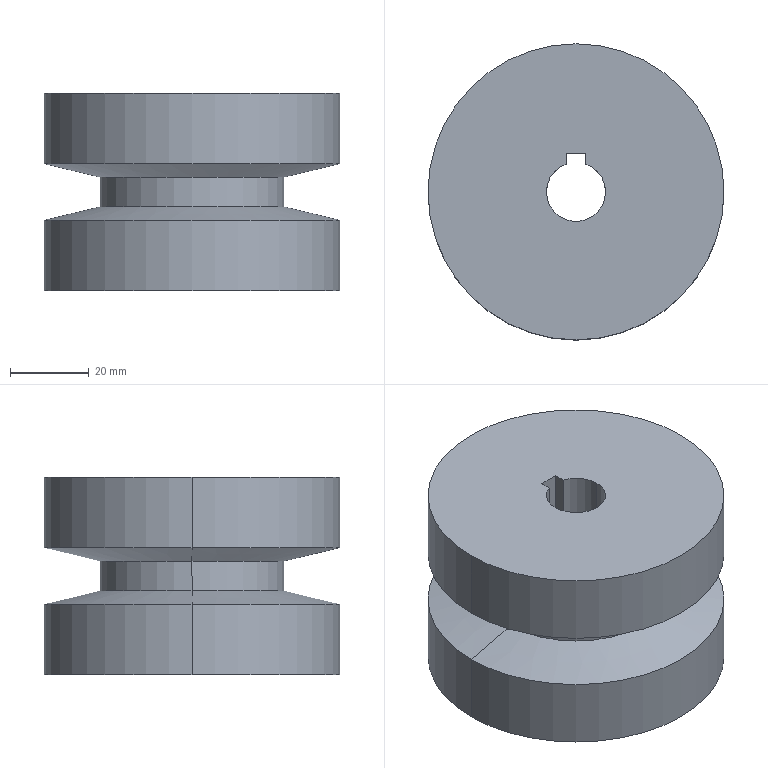Part | SolidWorks | features HoleWzd 2, Extrusion 1, ICE 1, RevCut 1 | 1 solid | 24 faces | box 75 x 75 x 50 mm | volume 180356 mm3 | cylinder 13 | plane 7 | cone 4 | commonest cylinder face diameters 4.2 x4 75 x4 15 x3 46.5 x2
STEP:
#1=CARTESIAN_POINT('',(0.,9.8,11.1));
#2=VERTEX_POINT('',#1);
#3=CARTESIAN_POINT('',(0.,9.8,6.9));
#4=VERTEX_POINT('',#3);
#5=CARTESIAN_POINT('',(0.,9.8,9.));
#6=DIRECTION('',(0.,-1.,0.));
#7=DIRECTION('',(0.,0.,1.));
#8=AXIS2_PLACEMENT_3D('',#5,#6,#7);
#9=CIRCLE('',#8,2.1);
#10=EDGE_CURVE('',#2,#4,#9,.T.);
#11=ORIENTED_EDGE('',*,*,#10,.T.);
#12=CARTESIAN_POINT('',(0.,32.5,6.9));
#13=VERTEX_POINT('',#12);
#14=CARTESIAN_POINT('',(0.,32.5,6.9));
#15=DIRECTION('',(0.,1.,0.));
#16=VECTOR('',#15,1000.);
#17=LINE('',#14,#16);
#18=EDGE_CURVE('',#4,#13,#17,.T.);
#19=ORIENTED_EDGE('',*,*,#18,.T.);
#20=CARTESIAN_POINT('',(0.,32.5,11.1));
#21=VERTEX_POINT('',#20);
#22=CARTESIAN_POINT('',(0.,32.5,9.));
#23=DIRECTION('',(0.,1.,0.));
#24=DIRECTION('',(0.,0.,1.));
#25=AXIS2_PLACEMENT_3D('',#22,#23,#24);
#26=CIRCLE('',#25,2.1);
#27=EDGE_CURVE('',#13,#21,#26,.T.);
#28=ORIENTED_EDGE('',*,*,#27,.T.);
#29=CARTESIAN_POINT('',(0.,32.5,11.1));
#30=DIRECTION('',(0.,1.,0.));
#31=VECTOR('',#30,1000.);
#32=LINE('',#29,#31);
#33=EDGE_CURVE('',#2,#21,#32,.T.);
#34=ORIENTED_EDGE('',*,*,#33,.F.);
#35=EDGE_LOOP('',(#11,#19,#28,#34));
#36=FACE_OUTER_BOUND('',#35,.T.);
#37=CARTESIAN_POINT('',(0.,32.5,9.));
#38=DIRECTION('',(0.,1.,0.));
#39=DIRECTION('',(0.,0.,1.));
#40=AXIS2_PLACEMENT_3D('',#37,#38,#39);
#41=CYLINDRICAL_SURFACE('',#40,2.1);
#42=ADVANCED_FACE('',(#36),#41,.F.);
#43=CARTESIAN_POINT('',(7.5,0.,6.9));
#44=VERTEX_POINT('',#43);
#45=CARTESIAN_POINT('',(7.5,0.,11.1));
#46=VERTEX_POINT('',#45);
#47=CARTESIAN_POINT('',(7.5,0.,6.9));
#48=CARTESIAN_POINT('',(7.5,-0.1395,6.9));
#49=CARTESIAN_POINT('',(7.496,-0.2765,6.914));
#50=CARTESIAN_POINT('',(7.481,-0.5459,6.968));
#51=CARTESIAN_POINT('',(7.47,-0.6797,7.008));
#52=CARTESIAN_POINT('',(7.443,-0.9337,7.114));
#53=CARTESIAN_POINT('',(7.426,-1.054,7.179));
#54=CARTESIAN_POINT('',(7.391,-1.282,7.331));
#55=CARTESIAN_POINT('',(7.371,-1.389,7.419));
#56=CARTESIAN_POINT('',(7.313,-1.678,7.708));
#57=CARTESIAN_POINT('',(7.273,-1.834,7.941));
#58=CARTESIAN_POINT('',(7.231,-1.992,8.32));
#59=CARTESIAN_POINT('',(7.219,-2.032,8.453));
#60=CARTESIAN_POINT('',(7.204,-2.086,8.725));
#61=CARTESIAN_POINT('',(7.2,-2.1,8.861));
#62=CARTESIAN_POINT('',(7.2,-2.1,9.137));
#63=CARTESIAN_POINT('',(7.204,-2.086,9.277));
#64=CARTESIAN_POINT('',(7.219,-2.032,9.547));
#65=CARTESIAN_POINT('',(7.231,-1.992,9.678));
#66=CARTESIAN_POINT('',(7.273,-1.833,10.061));
#67=CARTESIAN_POINT('',(7.312,-1.679,10.291));
#68=CARTESIAN_POINT('',(7.371,-1.387,10.582));
#69=CARTESIAN_POINT('',(7.39,-1.282,10.669));
#70=CARTESIAN_POINT('',(7.426,-1.055,10.821));
#71=CARTESIAN_POINT('',(7.443,-0.9321,10.887));
#72=CARTESIAN_POINT('',(7.47,-0.6788,10.992));
#73=CARTESIAN_POINT('',(7.481,-0.5478,11.032));
#74=CARTESIAN_POINT('',(7.496,-0.2769,11.086));
#75=CARTESIAN_POINT('',(7.5,-0.1375,11.1));
#76=CARTESIAN_POINT('',(7.5,0.,11.1));
#77=B_SPLINE_CURVE_WITH_KNOTS('',3,(#47,#48,#49,#50,#51,#52,#53,#54,#55,#56,#57,#58,#59,#60,#61,#62,#63,#64,#65,#66,#67,#68,#69,#70,#71,#72,#73,#74,#75,#76),.UNSPECIFIED.,.F.,.F.,(4,2,2,2,2,2,2,2,2,2,2,2,2,2,4),(0.,0.0004124,0.0008248,0.001237,0.00165,0.002475,0.002887,0.003299,0.003712,0.004124,0.004949,0.005361,0.005774,0.006186,0.006599),.UNSPECIFIED.);
#78=EDGE_CURVE('',#44,#46,#77,.T.);
#79=ORIENTED_EDGE('',*,*,#78,.T.);
#80=CARTESIAN_POINT('',(32.5,0.,11.1));
#81=VERTEX_POINT('',#80);
#82=CARTESIAN_POINT('',(32.5,0.,11.1));
#83=DIRECTION('',(1.,0.,0.));
#84=VECTOR('',#83,1000.);
#85=LINE('',#82,#84);
#86=EDGE_CURVE('',#46,#81,#85,.T.);
#87=ORIENTED_EDGE('',*,*,#86,.T.);
#88=CARTESIAN_POINT('',(32.5,0.,6.9));
#89=VERTEX_POINT('',#88);
#90=CARTESIAN_POINT('',(32.5,0.,9.));
#91=DIRECTION('',(1.,0.,0.));
#92=DIRECTION('',(0.,0.,-1.));
#93=AXIS2_PLACEMENT_3D('',#90,#91,#92);
#94=CIRCLE('',#93,2.1);
#95=EDGE_CURVE('',#81,#89,#94,.T.);
#96=ORIENTED_EDGE('',*,*,#95,.T.);
#97=CARTESIAN_POINT('',(32.5,0.,6.9));
#98=DIRECTION('',(1.,0.,0.));
#99=VECTOR('',#98,1000.);
#100=LINE('',#97,#99);
#101=EDGE_CURVE('',#44,#89,#100,.T.);
#102=ORIENTED_EDGE('',*,*,#101,.F.);
#103=EDGE_LOOP('',(#79,#87,#96,#102));
#104=FACE_OUTER_BOUND('',#103,.T.);
#105=CARTESIAN_POINT('',(32.5,0.,9.));
#106=DIRECTION('',(1.,0.,0.));
#107=DIRECTION('',(0.,0.,-1.));
#108=AXIS2_PLACEMENT_3D('',#105,#106,#107);
#109=CYLINDRICAL_SURFACE('',#108,2.1);
#110=ADVANCED_FACE('',(#104),#109,.F.);
#111=CARTESIAN_POINT('',(-23.25,0.,28.75));
#112=VERTEX_POINT('',#111);
#113=CARTESIAN_POINT('',(23.25,0.,28.75));
#114=VERTEX_POINT('',#113);
#115=CARTESIAN_POINT('',(0.,0.,28.75));
#116=DIRECTION('',(0.,0.,-1.));
#117=DIRECTION('',(-1.,0.,0.));
#118=AXIS2_PLACEMENT_3D('',#115,#116,#117);
#119=CIRCLE('',#118,23.25);
#120=EDGE_CURVE('',#112,#114,#119,.T.);
#121=ORIENTED_EDGE('',*,*,#120,.T.);
#122=CARTESIAN_POINT('',(23.25,0.,21.25));
#123=VERTEX_POINT('',#122);
#124=CARTESIAN_POINT('',(23.25,0.,0.));
#125=DIRECTION('',(0.,0.,-1.));
#126=VECTOR('',#125,1000.);
#127=LINE('',#124,#126);
#128=EDGE_CURVE('',#114,#123,#127,.T.);
#129=ORIENTED_EDGE('',*,*,#128,.T.);
#130=CARTESIAN_POINT('',(-23.25,0.,21.25));
#131=VERTEX_POINT('',#130);
#132=CARTESIAN_POINT('',(0.,0.,21.25));
#133=DIRECTION('',(0.,0.,-1.));
#134=DIRECTION('',(-1.,0.,0.));
#135=AXIS2_PLACEMENT_3D('',#132,#133,#134);
#136=CIRCLE('',#135,23.25);
#137=EDGE_CURVE('',#131,#123,#136,.T.);
#138=ORIENTED_EDGE('',*,*,#137,.F.);
#139=CARTESIAN_POINT('',(-23.25,0.,0.));
#140=DIRECTION('',(0.,0.,-1.));
#141=VECTOR('',#140,1000.);
#142=LINE('',#139,#141);
#143=EDGE_CURVE('',#112,#131,#142,.T.);
#144=ORIENTED_EDGE('',*,*,#143,.F.);
#145=EDGE_LOOP('',(#121,#129,#138,#144));
#146=FACE_OUTER_BOUND('',#145,.T.);
#147=CARTESIAN_POINT('',(0.,0.,0.));
#148=DIRECTION('',(0.,0.,-1.));
#149=DIRECTION('',(-1.,0.,0.));
#150=AXIS2_PLACEMENT_3D('',#147,#148,#149);
#151=CYLINDRICAL_SURFACE('',#150,23.25);
#152=ADVANCED_FACE('',(#146),#151,.T.);
#153=ORIENTED_EDGE('',*,*,#120,.F.);
#154=CARTESIAN_POINT('',(-37.5,0.,32.171));
#155=VERTEX_POINT('',#154);
#156=CARTESIAN_POINT('',(-38.25,0.,32.351));
#157=DIRECTION('',(-0.9724,0.,0.2334));
#158=VECTOR('',#157,1000.);
#159=LINE('',#156,#158);
#160=EDGE_CURVE('',#112,#155,#159,.T.);
#161=ORIENTED_EDGE('',*,*,#160,.T.);
#162=CARTESIAN_POINT('',(37.5,0.,32.171));
#163=VERTEX_POINT('',#162);
#164=CARTESIAN_POINT('',(0.,0.,32.171));
#165=DIRECTION('',(0.,0.,1.));
#166=DIRECTION('',(1.,0.,0.));
#167=AXIS2_PLACEMENT_3D('',#164,#165,#166);
#168=CIRCLE('',#167,37.5);
#169=EDGE_CURVE('',#163,#155,#168,.T.);
#170=ORIENTED_EDGE('',*,*,#169,.F.);
#171=CARTESIAN_POINT('',(38.25,0.,32.351));
#172=DIRECTION('',(0.9724,0.,0.2334));
#173=VECTOR('',#172,1000.);
#174=LINE('',#171,#173);
#175=EDGE_CURVE('',#114,#163,#174,.T.);
#176=ORIENTED_EDGE('',*,*,#175,.F.);
#177=EDGE_LOOP('',(#153,#161,#170,#176));
#178=FACE_OUTER_BOUND('',#177,.T.);
#179=CARTESIAN_POINT('',(0.,0.,32.351));
#180=DIRECTION('',(0.,0.,1.));
#181=DIRECTION('',(1.,0.,0.));
#182=AXIS2_PLACEMENT_3D('',#179,#180,#181);
#183=CONICAL_SURFACE('',#182,38.25,1.335);
#184=ADVANCED_FACE('',(#178),#183,.T.);
#185=ORIENTED_EDGE('',*,*,#137,.T.);
#186=CARTESIAN_POINT('',(37.5,0.,17.829));
#187=VERTEX_POINT('',#186);
#188=CARTESIAN_POINT('',(23.25,0.,21.25));
#189=DIRECTION('',(0.9724,0.,-0.2334));
#190=VECTOR('',#189,1000.);
#191=LINE('',#188,#190);
#192=EDGE_CURVE('',#123,#187,#191,.T.);
#193=ORIENTED_EDGE('',*,*,#192,.T.);
#194=CARTESIAN_POINT('',(-37.5,0.,17.829));
#195=VERTEX_POINT('',#194);
#196=CARTESIAN_POINT('',(0.,0.,17.829));
#197=DIRECTION('',(0.,0.,-1.));
#198=DIRECTION('',(-1.,0.,0.));
#199=AXIS2_PLACEMENT_3D('',#196,#197,#198);
#200=CIRCLE('',#199,37.5);
#201=EDGE_CURVE('',#195,#187,#200,.T.);
#202=ORIENTED_EDGE('',*,*,#201,.F.);
#203=CARTESIAN_POINT('',(-23.25,0.,21.25));
#204=DIRECTION('',(-0.9724,0.,-0.2334));
#205=VECTOR('',#204,1000.);
#206=LINE('',#203,#205);
#207=EDGE_CURVE('',#131,#195,#206,.T.);
#208=ORIENTED_EDGE('',*,*,#207,.F.);
#209=EDGE_LOOP('',(#185,#193,#202,#208));
#210=FACE_OUTER_BOUND('',#209,.T.);
#211=CARTESIAN_POINT('',(0.,0.,21.25));
#212=DIRECTION('',(0.,0.,-1.));
#213=DIRECTION('',(-1.,0.,0.));
#214=AXIS2_PLACEMENT_3D('',#211,#212,#213);
#215=CONICAL_SURFACE('',#214,23.25,1.335);
#216=ADVANCED_FACE('',(#210),#215,.T.);
#217=CARTESIAN_POINT('',(-7.5,0.,50.));
#218=VERTEX_POINT('',#217);
#219=CARTESIAN_POINT('',(7.5,0.,50.));
#220=VERTEX_POINT('',#219);
#221=CARTESIAN_POINT('',(0.,0.,50.));
#222=DIRECTION('',(0.,0.,1.));
#223=DIRECTION('',(1.,0.,0.));
#224=AXIS2_PLACEMENT_3D('',#221,#222,#223);
#225=CIRCLE('',#224,7.5);
#226=EDGE_CURVE('',#218,#220,#225,.T.);
#227=ORIENTED_EDGE('',*,*,#226,.T.);
#228=CARTESIAN_POINT('',(7.5,0.,50.));
#229=DIRECTION('',(0.,0.,-1.));
#230=VECTOR('',#229,1000.);
#231=LINE('',#228,#230);
#232=EDGE_CURVE('',#220,#46,#231,.T.);
#233=ORIENTED_EDGE('',*,*,#232,.T.);
#234=ORIENTED_EDGE('',*,*,#78,.F.);
#235=CARTESIAN_POINT('',(7.5,0.,0.));
#236=VERTEX_POINT('',#235);
#237=CARTESIAN_POINT('',(7.5,0.,50.));
#238=DIRECTION('',(0.,0.,-1.));
#239=VECTOR('',#238,1000.);
#240=LINE('',#237,#239);
#241=EDGE_CURVE('',#44,#236,#240,.T.);
#242=ORIENTED_EDGE('',*,*,#241,.T.);
#243=CARTESIAN_POINT('',(-7.5,0.,0.));
#244=VERTEX_POINT('',#243);
#245=CARTESIAN_POINT('',(0.,0.,0.));
#246=DIRECTION('',(0.,0.,1.));
#247=DIRECTION('',(1.,0.,0.));
#248=AXIS2_PLACEMENT_3D('',#245,#246,#247);
#249=CIRCLE('',#248,7.5);
#250=EDGE_CURVE('',#244,#236,#249,.T.);
#251=ORIENTED_EDGE('',*,*,#250,.F.);
#252=CARTESIAN_POINT('',(-7.5,0.,50.));
#253=DIRECTION('',(0.,0.,-1.));
#254=VECTOR('',#253,1000.);
#255=LINE('',#252,#254);
#256=EDGE_CURVE('',#218,#244,#255,.T.);
#257=ORIENTED_EDGE('',*,*,#256,.F.);
#258=EDGE_LOOP('',(#227,#233,#234,#242,#251,#257));
#259=FACE_OUTER_BOUND('',#258,.T.);
#260=CARTESIAN_POINT('',(0.,0.,50.));
#261=DIRECTION('',(0.,0.,-1.));
#262=DIRECTION('',(-1.,0.,0.));
#263=AXIS2_PLACEMENT_3D('',#260,#261,#262);
#264=CYLINDRICAL_SURFACE('',#263,7.5);
#265=ADVANCED_FACE('',(#259),#264,.F.);
#266=CARTESIAN_POINT('',(-2.5,7.071,50.));
#267=VERTEX_POINT('',#266);
#268=CARTESIAN_POINT('',(0.,0.,50.));
#269=DIRECTION('',(0.,0.,1.));
#270=DIRECTION('',(1.,0.,0.));
#271=AXIS2_PLACEMENT_3D('',#268,#269,#270);
#272=CIRCLE('',#271,7.5);
#273=EDGE_CURVE('',#267,#218,#272,.T.);
#274=ORIENTED_EDGE('',*,*,#273,.T.);
#275=ORIENTED_EDGE('',*,*,#256,.T.);
#276=CARTESIAN_POINT('',(-2.5,7.071,0.));
#277=VERTEX_POINT('',#276);
#278=CARTESIAN_POINT('',(0.,0.,0.));
#279=DIRECTION('',(0.,0.,1.));
#280=DIRECTION('',(1.,0.,0.));
#281=AXIS2_PLACEMENT_3D('',#278,#279,#280);
#282=CIRCLE('',#281,7.5);
#283=EDGE_CURVE('',#277,#244,#282,.T.);
#284=ORIENTED_EDGE('',*,*,#283,.F.);
#285=CARTESIAN_POINT('',(-2.5,7.071,50.));
#286=DIRECTION('',(0.,0.,-1.));
#287=VECTOR('',#286,1000.);
#288=LINE('',#285,#287);
#289=EDGE_CURVE('',#267,#277,#288,.T.);
#290=ORIENTED_EDGE('',*,*,#289,.F.);
#291=EDGE_LOOP('',(#274,#275,#284,#290));
#292=FACE_OUTER_BOUND('',#291,.T.);
#293=CARTESIAN_POINT('',(0.,0.,50.));
#294=DIRECTION('',(0.,0.,-1.));
#295=DIRECTION('',(-1.,0.,0.));
#296=AXIS2_PLACEMENT_3D('',#293,#294,#295);
#297=CYLINDRICAL_SURFACE('',#296,7.5);
#298=ADVANCED_FACE('',(#292),#297,.F.);
#299=CARTESIAN_POINT('',(37.5,0.,50.));
#300=VERTEX_POINT('',#299);
#301=CARTESIAN_POINT('',(-37.5,0.,50.));
#302=VERTEX_POINT('',#301);
#303=CARTESIAN_POINT('',(0.,0.,50.));
#304=DIRECTION('',(0.,0.,1.));
#305=DIRECTION('',(1.,0.,0.));
#306=AXIS2_PLACEMENT_3D('',#303,#304,#305);
#307=CIRCLE('',#306,37.5);
#308=EDGE_CURVE('',#300,#302,#307,.T.);
#309=ORIENTED_EDGE('',*,*,#308,.F.);
#310=CARTESIAN_POINT('',(37.5,0.,50.));
#311=DIRECTION('',(0.,0.,-1.));
#312=VECTOR('',#311,1000.);
#313=LINE('',#310,#312);
#314=EDGE_CURVE('',#300,#163,#313,.T.);
#315=ORIENTED_EDGE('',*,*,#314,.T.);
#316=ORIENTED_EDGE('',*,*,#169,.T.);
#317=CARTESIAN_POINT('',(-37.5,0.,50.));
#318=DIRECTION('',(0.,0.,-1.));
#319=VECTOR('',#318,1000.);
#320=LINE('',#317,#319);
#321=EDGE_CURVE('',#302,#155,#320,.T.);
#322=ORIENTED_EDGE('',*,*,#321,.F.);
#323=EDGE_LOOP('',(#309,#315,#316,#322));
#324=FACE_OUTER_BOUND('',#323,.T.);
#325=CARTESIAN_POINT('',(0.,0.,50.));
#326=DIRECTION('',(0.,0.,-1.));
#327=DIRECTION('',(-1.,0.,0.));
#328=AXIS2_PLACEMENT_3D('',#325,#326,#327);
#329=CYLINDRICAL_SURFACE('',#328,37.5);
#330=ADVANCED_FACE('',(#324),#329,.T.);
#331=ORIENTED_EDGE('',*,*,#201,.T.);
#332=CARTESIAN_POINT('',(37.5,0.,0.));
#333=VERTEX_POINT('',#332);
#334=CARTESIAN_POINT('',(37.5,0.,50.));
#335=DIRECTION('',(0.,0.,-1.));
#336=VECTOR('',#335,1000.);
#337=LINE('',#334,#336);
#338=EDGE_CURVE('',#187,#333,#337,.T.);
#339=ORIENTED_EDGE('',*,*,#338,.T.);
#340=CARTESIAN_POINT('',(-37.5,0.,0.));
#341=VERTEX_POINT('',#340);
#342=CARTESIAN_POINT('',(0.,0.,0.));
#343=DIRECTION('',(0.,0.,1.));
#344=DIRECTION('',(1.,0.,0.));
#345=AXIS2_PLACEMENT_3D('',#342,#343,#344);
#346=CIRCLE('',#345,37.5);
#347=EDGE_CURVE('',#333,#341,#346,.T.);
#348=ORIENTED_EDGE('',*,*,#347,.T.);
#349=CARTESIAN_POINT('',(-37.5,0.,50.));
#350=DIRECTION('',(0.,0.,-1.));
#351=VECTOR('',#350,1000.);
#352=LINE('',#349,#351);
#353=EDGE_CURVE('',#195,#341,#352,.T.);
#354=ORIENTED_EDGE('',*,*,#353,.F.);
#355=EDGE_LOOP('',(#331,#339,#348,#354));
#356=FACE_OUTER_BOUND('',#355,.T.);
#357=CARTESIAN_POINT('',(0.,0.,50.));
#358=DIRECTION('',(0.,0.,-1.));
#359=DIRECTION('',(-1.,0.,0.));
#360=AXIS2_PLACEMENT_3D('',#357,#358,#359);
#361=CYLINDRICAL_SURFACE('',#360,37.5);
#362=ADVANCED_FACE('',(#356),#361,.T.);
#363=ORIENTED_EDGE('',*,*,#338,.F.);
#364=CARTESIAN_POINT('',(0.,0.,17.829));
#365=DIRECTION('',(0.,0.,-1.));
#366=DIRECTION('',(-1.,0.,0.));
#367=AXIS2_PLACEMENT_3D('',#364,#365,#366);
#368=CIRCLE('',#367,37.5);
#369=EDGE_CURVE('',#187,#195,#368,.T.);
#370=ORIENTED_EDGE('',*,*,#369,.T.);
#371=ORIENTED_EDGE('',*,*,#353,.T.);
#372=CARTESIAN_POINT('',(0.,0.,0.));
#373=DIRECTION('',(0.,0.,1.));
#374=DIRECTION('',(1.,0.,0.));
#375=AXIS2_PLACEMENT_3D('',#372,#373,#374);
#376=CIRCLE('',#375,37.5);
#377=EDGE_CURVE('',#341,#333,#376,.T.);
#378=ORIENTED_EDGE('',*,*,#377,.T.);
#379=EDGE_LOOP('',(#363,#370,#371,#378));
#380=FACE_OUTER_BOUND('',#379,.T.);
#381=CARTESIAN_POINT('',(0.,0.,50.));
#382=DIRECTION('',(0.,0.,-1.));
#383=DIRECTION('',(-1.,0.,0.));
#384=AXIS2_PLACEMENT_3D('',#381,#382,#383);
#385=CYLINDRICAL_SURFACE('',#384,37.5);
#386=ADVANCED_FACE('',(#380),#385,.T.);
#387=CARTESIAN_POINT('',(-2.5,9.8,50.));
#388=VERTEX_POINT('',#387);
#389=CARTESIAN_POINT('',(-2.5,0.,50.));
#390=DIRECTION('',(0.,-1.,0.));
#391=VECTOR('',#390,1000.);
#392=LINE('',#389,#391);
#393=EDGE_CURVE('',#388,#267,#392,.T.);
#394=ORIENTED_EDGE('',*,*,#393,.F.);
#395=CARTESIAN_POINT('',(2.5,9.8,50.));
#396=VERTEX_POINT('',#395);
#397=CARTESIAN_POINT('',(0.,9.8,50.));
#398=DIRECTION('',(-1.,0.,0.));
#399=VECTOR('',#398,1000.);
#400=LINE('',#397,#399);
#401=EDGE_CURVE('',#396,#388,#400,.T.);
#402=ORIENTED_EDGE('',*,*,#401,.F.);
#403=CARTESIAN_POINT('',(2.5,7.071,50.));
#404=VERTEX_POINT('',#403);
#405=CARTESIAN_POINT('',(2.5,0.,50.));
#406=DIRECTION('',(0.,1.,0.));
#407=VECTOR('',#406,1000.);
#408=LINE('',#405,#407);
#409=EDGE_CURVE('',#404,#396,#408,.T.);
#410=ORIENTED_EDGE('',*,*,#409,.F.);
#411=CARTESIAN_POINT('',(0.,0.,50.));
#412=DIRECTION('',(0.,0.,1.));
#413=DIRECTION('',(1.,0.,0.));
#414=AXIS2_PLACEMENT_3D('',#411,#412,#413);
#415=CIRCLE('',#414,7.5);
#416=EDGE_CURVE('',#220,#404,#415,.T.);
#417=ORIENTED_EDGE('',*,*,#416,.F.);
#418=ORIENTED_EDGE('',*,*,#226,.F.);
#419=ORIENTED_EDGE('',*,*,#273,.F.);
#420=EDGE_LOOP('',(#394,#402,#410,#417,#418,#419));
#421=FACE_BOUND('',#420,.T.);
#422=CARTESIAN_POINT('',(0.,0.,50.));
#423=DIRECTION('',(0.,0.,1.));
#424=DIRECTION('',(1.,0.,0.));
#425=AXIS2_PLACEMENT_3D('',#422,#423,#424);
#426=CIRCLE('',#425,37.5);
#427=EDGE_CURVE('',#302,#300,#426,.T.);
#428=ORIENTED_EDGE('',*,*,#427,.T.);
#429=ORIENTED_EDGE('',*,*,#308,.T.);
#430=EDGE_LOOP('',(#428,#429));
#431=FACE_OUTER_BOUND('',#430,.T.);
#432=CARTESIAN_POINT('',(0.,0.,50.));
#433=DIRECTION('',(0.,0.,1.));
#434=DIRECTION('',(1.,0.,0.));
#435=AXIS2_PLACEMENT_3D('',#432,#433,#434);
#436=PLANE('',#435);
#437=ADVANCED_FACE('',(#421,#431),#436,.T.);
#438=ORIENTED_EDGE('',*,*,#377,.F.);
#439=ORIENTED_EDGE('',*,*,#347,.F.);
#440=EDGE_LOOP('',(#438,#439));
#441=FACE_OUTER_BOUND('',#440,.T.);
#442=CARTESIAN_POINT('',(-2.5,9.8,0.));
#443=VERTEX_POINT('',#442);
#444=CARTESIAN_POINT('',(2.5,9.8,0.));
#445=VERTEX_POINT('',#444);
#446=CARTESIAN_POINT('',(2.5,9.8,0.));
#447=DIRECTION('',(1.,0.,0.));
#448=VECTOR('',#447,1000.);
#449=LINE('',#446,#448);
#450=EDGE_CURVE('',#443,#445,#449,.T.);
#451=ORIENTED_EDGE('',*,*,#450,.F.);
#452=CARTESIAN_POINT('',(-2.5,5.2,0.));
#453=DIRECTION('',(0.,1.,0.));
#454=VECTOR('',#453,1000.);
#455=LINE('',#452,#454);
#456=EDGE_CURVE('',#277,#443,#455,.T.);
#457=ORIENTED_EDGE('',*,*,#456,.F.);
#458=ORIENTED_EDGE('',*,*,#283,.T.);
#459=ORIENTED_EDGE('',*,*,#250,.T.);
#460=CARTESIAN_POINT('',(2.5,7.071,0.));
#461=VERTEX_POINT('',#460);
#462=CARTESIAN_POINT('',(0.,0.,0.));
#463=DIRECTION('',(0.,0.,1.));
#464=DIRECTION('',(1.,0.,0.));
#465=AXIS2_PLACEMENT_3D('',#462,#463,#464);
#466=CIRCLE('',#465,7.5);
#467=EDGE_CURVE('',#236,#461,#466,.T.);
#468=ORIENTED_EDGE('',*,*,#467,.T.);
#469=CARTESIAN_POINT('',(2.5,5.2,0.));
#470=DIRECTION('',(0.,-1.,0.));
#471=VECTOR('',#470,1000.);
#472=LINE('',#469,#471);
#473=EDGE_CURVE('',#445,#461,#472,.T.);
#474=ORIENTED_EDGE('',*,*,#473,.F.);
#475=EDGE_LOOP('',(#451,#457,#458,#459,#468,#474));
#476=FACE_BOUND('',#475,.T.);
#477=CARTESIAN_POINT('',(0.,0.,0.));
#478=DIRECTION('',(0.,0.,1.));
#479=DIRECTION('',(1.,0.,0.));
#480=AXIS2_PLACEMENT_3D('',#477,#478,#479);
#481=PLANE('',#480);
#482=ADVANCED_FACE('',(#441,#476),#481,.F.);
#483=ORIENTED_EDGE('',*,*,#314,.F.);
#484=ORIENTED_EDGE('',*,*,#427,.F.);
#485=ORIENTED_EDGE('',*,*,#321,.T.);
#486=CARTESIAN_POINT('',(0.,0.,32.171));
#487=DIRECTION('',(0.,0.,1.));
#488=DIRECTION('',(1.,0.,0.));
#489=AXIS2_PLACEMENT_3D('',#486,#487,#488);
#490=CIRCLE('',#489,37.5);
#491=EDGE_CURVE('',#155,#163,#490,.T.);
#492=ORIENTED_EDGE('',*,*,#491,.T.);
#493=EDGE_LOOP('',(#483,#484,#485,#492));
#494=FACE_OUTER_BOUND('',#493,.T.);
#495=CARTESIAN_POINT('',(0.,0.,50.));
#496=DIRECTION('',(0.,0.,-1.));
#497=DIRECTION('',(-1.,0.,0.));
#498=AXIS2_PLACEMENT_3D('',#495,#496,#497);
#499=CYLINDRICAL_SURFACE('',#498,37.5);
#500=ADVANCED_FACE('',(#494),#499,.T.);
#501=ORIENTED_EDGE('',*,*,#232,.F.);
#502=ORIENTED_EDGE('',*,*,#416,.T.);
#503=CARTESIAN_POINT('',(2.5,7.071,50.));
#504=DIRECTION('',(0.,0.,1.));
#505=VECTOR('',#504,1000.);
#506=LINE('',#503,#505);
#507=EDGE_CURVE('',#461,#404,#506,.T.);
#508=ORIENTED_EDGE('',*,*,#507,.F.);
#509=ORIENTED_EDGE('',*,*,#467,.F.);
#510=ORIENTED_EDGE('',*,*,#241,.F.);
#511=CARTESIAN_POINT('',(7.5,0.,11.1));
#512=CARTESIAN_POINT('',(7.5,0.2749,11.1));
#513=CARTESIAN_POINT('',(7.484,0.5525,11.044));
#514=CARTESIAN_POINT('',(7.443,0.9321,10.887));
#515=CARTESIAN_POINT('',(7.426,1.055,10.821));
#516=CARTESIAN_POINT('',(7.39,1.282,10.669));
#517=CARTESIAN_POINT('',(7.371,1.388,10.582));
#518=CARTESIAN_POINT('',(7.332,1.581,10.388));
#519=CARTESIAN_POINT('',(7.312,1.669,10.281));
#520=CARTESIAN_POINT('',(7.276,1.821,10.055));
#521=CARTESIAN_POINT('',(7.259,1.886,9.934));
#522=CARTESIAN_POINT('',(7.231,1.992,9.679));
#523=CARTESIAN_POINT('',(7.219,2.032,9.547));
#524=CARTESIAN_POINT('',(7.204,2.086,9.278));
#525=CARTESIAN_POINT('',(7.2,2.1,9.139));
#526=CARTESIAN_POINT('',(7.2,2.1,8.862));
#527=CARTESIAN_POINT('',(7.204,2.086,8.725));
#528=CARTESIAN_POINT('',(7.219,2.033,8.455));
#529=CARTESIAN_POINT('',(7.231,1.992,8.321));
#530=CARTESIAN_POINT('',(7.273,1.834,7.941));
#531=CARTESIAN_POINT('',(7.312,1.678,7.708));
#532=CARTESIAN_POINT('',(7.371,1.389,7.419));
#533=CARTESIAN_POINT('',(7.39,1.283,7.331));
#534=CARTESIAN_POINT('',(7.426,1.054,7.179));
#535=CARTESIAN_POINT('',(7.443,0.9341,7.114));
#536=CARTESIAN_POINT('',(7.47,0.6811,7.009));
#537=CARTESIAN_POINT('',(7.481,0.5471,6.968));
#538=CARTESIAN_POINT('',(7.496,0.2768,6.914));
#539=CARTESIAN_POINT('',(7.5,0.1395,6.9));
#540=CARTESIAN_POINT('',(7.5,0.,6.9));
#541=B_SPLINE_CURVE_WITH_KNOTS('',3,(#511,#512,#513,#514,#515,#516,#517,#518,#519,#520,#521,#522,#523,#524,#525,#526,#527,#528,#529,#530,#531,#532,#533,#534,#535,#536,#537,#538,#539,#540),.UNSPECIFIED.,.F.,.F.,(4,2,2,2,2,2,2,2,2,2,2,2,2,2,4),(0.006599,0.007423,0.007836,0.008248,0.00866,0.009073,0.009485,0.009897,0.01031,0.01072,0.01155,0.01196,0.01237,0.01278,0.0132),.UNSPECIFIED.);
#542=EDGE_CURVE('',#46,#44,#541,.T.);
#543=ORIENTED_EDGE('',*,*,#542,.F.);
#544=EDGE_LOOP('',(#501,#502,#508,#509,#510,#543));
#545=FACE_OUTER_BOUND('',#544,.T.);
#546=CARTESIAN_POINT('',(0.,0.,50.));
#547=DIRECTION('',(0.,0.,-1.));
#548=DIRECTION('',(-1.,0.,0.));
#549=AXIS2_PLACEMENT_3D('',#546,#547,#548);
#550=CYLINDRICAL_SURFACE('',#549,7.5);
#551=ADVANCED_FACE('',(#545),#550,.F.);
#552=ORIENTED_EDGE('',*,*,#192,.F.);
#553=CARTESIAN_POINT('',(0.,0.,21.25));
#554=DIRECTION('',(0.,0.,-1.));
#555=DIRECTION('',(-1.,0.,0.));
#556=AXIS2_PLACEMENT_3D('',#553,#554,#555);
#557=CIRCLE('',#556,23.25);
#558=EDGE_CURVE('',#123,#131,#557,.T.);
#559=ORIENTED_EDGE('',*,*,#558,.T.);
#560=ORIENTED_EDGE('',*,*,#207,.T.);
#561=ORIENTED_EDGE('',*,*,#369,.F.);
#562=EDGE_LOOP('',(#552,#559,#560,#561));
#563=FACE_OUTER_BOUND('',#562,.T.);
#564=CARTESIAN_POINT('',(0.,0.,21.25));
#565=DIRECTION('',(0.,0.,-1.));
#566=DIRECTION('',(-1.,0.,0.));
#567=AXIS2_PLACEMENT_3D('',#564,#565,#566);
#568=CONICAL_SURFACE('',#567,23.25,1.335);
#569=ADVANCED_FACE('',(#563),#568,.T.);
#570=ORIENTED_EDGE('',*,*,#160,.F.);
#571=CARTESIAN_POINT('',(0.,0.,28.75));
#572=DIRECTION('',(0.,0.,-1.));
#573=DIRECTION('',(-1.,0.,0.));
#574=AXIS2_PLACEMENT_3D('',#571,#572,#573);
#575=CIRCLE('',#574,23.25);
#576=EDGE_CURVE('',#114,#112,#575,.T.);
#577=ORIENTED_EDGE('',*,*,#576,.F.);
#578=ORIENTED_EDGE('',*,*,#175,.T.);
#579=ORIENTED_EDGE('',*,*,#491,.F.);
#580=EDGE_LOOP('',(#570,#577,#578,#579));
#581=FACE_OUTER_BOUND('',#580,.T.);
#582=CARTESIAN_POINT('',(0.,0.,32.351));
#583=DIRECTION('',(0.,0.,1.));
#584=DIRECTION('',(1.,0.,0.));
#585=AXIS2_PLACEMENT_3D('',#582,#583,#584);
#586=CONICAL_SURFACE('',#585,38.25,1.335);
#587=ADVANCED_FACE('',(#581),#586,.T.);
#588=ORIENTED_EDGE('',*,*,#128,.F.);
#589=ORIENTED_EDGE('',*,*,#576,.T.);
#590=ORIENTED_EDGE('',*,*,#143,.T.);
#591=ORIENTED_EDGE('',*,*,#558,.F.);
#592=EDGE_LOOP('',(#588,#589,#590,#591));
#593=FACE_OUTER_BOUND('',#592,.T.);
#594=CARTESIAN_POINT('',(0.,0.,0.));
#595=DIRECTION('',(0.,0.,-1.));
#596=DIRECTION('',(-1.,0.,0.));
#597=AXIS2_PLACEMENT_3D('',#594,#595,#596);
#598=CYLINDRICAL_SURFACE('',#597,23.25);
#599=ADVANCED_FACE('',(#593),#598,.T.);
#600=CARTESIAN_POINT('',(32.5,0.,9.));
#601=DIRECTION('',(1.,0.,0.));
#602=DIRECTION('',(0.,0.,-1.));
#603=AXIS2_PLACEMENT_3D('',#600,#601,#602);
#604=CIRCLE('',#603,2.1);
#605=EDGE_CURVE('',#89,#81,#604,.T.);
#606=ORIENTED_EDGE('',*,*,#605,.F.);
#607=ORIENTED_EDGE('',*,*,#95,.F.);
#608=EDGE_LOOP('',(#606,#607));
#609=FACE_OUTER_BOUND('',#608,.T.);
#610=CARTESIAN_POINT('',(32.5,2.1,9.));
#611=DIRECTION('',(1.,0.,0.));
#612=DIRECTION('',(0.,0.,-1.));
#613=AXIS2_PLACEMENT_3D('',#610,#611,#612);
#614=PLANE('',#613);
#615=ADVANCED_FACE('',(#609),#614,.F.);
#616=ORIENTED_EDGE('',*,*,#86,.F.);
#617=ORIENTED_EDGE('',*,*,#542,.T.);
#618=ORIENTED_EDGE('',*,*,#101,.T.);
#619=ORIENTED_EDGE('',*,*,#605,.T.);
#620=EDGE_LOOP('',(#616,#617,#618,#619));
#621=FACE_OUTER_BOUND('',#620,.T.);
#622=CARTESIAN_POINT('',(32.5,0.,9.));
#623=DIRECTION('',(1.,0.,0.));
#624=DIRECTION('',(0.,0.,-1.));
#625=AXIS2_PLACEMENT_3D('',#622,#623,#624);
#626=CYLINDRICAL_SURFACE('',#625,2.1);
#627=ADVANCED_FACE('',(#621),#626,.F.);
#628=ORIENTED_EDGE('',*,*,#401,.T.);
#629=CARTESIAN_POINT('',(-2.5,9.8,90.));
#630=DIRECTION('',(0.,0.,-1.));
#631=VECTOR('',#630,1000.);
#632=LINE('',#629,#631);
#633=EDGE_CURVE('',#388,#443,#632,.T.);
#634=ORIENTED_EDGE('',*,*,#633,.T.);
#635=ORIENTED_EDGE('',*,*,#450,.T.);
#636=CARTESIAN_POINT('',(2.5,9.8,90.));
#637=DIRECTION('',(0.,0.,-1.));
#638=VECTOR('',#637,1000.);
#639=LINE('',#636,#638);
#640=EDGE_CURVE('',#396,#445,#639,.T.);
#641=ORIENTED_EDGE('',*,*,#640,.F.);
#642=EDGE_LOOP('',(#628,#634,#635,#641));
#643=FACE_OUTER_BOUND('',#642,.T.);
#644=ORIENTED_EDGE('',*,*,#10,.F.);
#645=CARTESIAN_POINT('',(0.,9.8,9.));
#646=DIRECTION('',(0.,-1.,0.));
#647=DIRECTION('',(0.,0.,1.));
#648=AXIS2_PLACEMENT_3D('',#645,#646,#647);
#649=CIRCLE('',#648,2.1);
#650=EDGE_CURVE('',#4,#2,#649,.T.);
#651=ORIENTED_EDGE('',*,*,#650,.F.);
#652=EDGE_LOOP('',(#644,#651));
#653=FACE_BOUND('',#652,.T.);
#654=CARTESIAN_POINT('',(2.5,9.8,90.));
#655=DIRECTION('',(0.,1.,0.));
#656=DIRECTION('',(0.,0.,1.));
#657=AXIS2_PLACEMENT_3D('',#654,#655,#656);
#658=PLANE('',#657);
#659=ADVANCED_FACE('',(#643,#653),#658,.F.);
#660=ORIENTED_EDGE('',*,*,#393,.T.);
#661=ORIENTED_EDGE('',*,*,#289,.T.);
#662=ORIENTED_EDGE('',*,*,#456,.T.);
#663=ORIENTED_EDGE('',*,*,#633,.F.);
#664=EDGE_LOOP('',(#660,#661,#662,#663));
#665=FACE_OUTER_BOUND('',#664,.T.);
#666=CARTESIAN_POINT('',(-2.5,5.2,90.));
#667=DIRECTION('',(-1.,0.,0.));
#668=DIRECTION('',(0.,0.,1.));
#669=AXIS2_PLACEMENT_3D('',#666,#667,#668);
#670=PLANE('',#669);
#671=ADVANCED_FACE('',(#665),#670,.F.);
#672=ORIENTED_EDGE('',*,*,#409,.T.);
#673=ORIENTED_EDGE('',*,*,#640,.T.);
#674=ORIENTED_EDGE('',*,*,#473,.T.);
#675=ORIENTED_EDGE('',*,*,#507,.T.);
#676=EDGE_LOOP('',(#672,#673,#674,#675));
#677=FACE_OUTER_BOUND('',#676,.T.);
#678=CARTESIAN_POINT('',(2.5,5.2,90.));
#679=DIRECTION('',(1.,0.,0.));
#680=DIRECTION('',(0.,0.,-1.));
#681=AXIS2_PLACEMENT_3D('',#678,#679,#680);
#682=PLANE('',#681);
#683=ADVANCED_FACE('',(#677),#682,.F.);
#684=CARTESIAN_POINT('',(0.,32.5,9.));
#685=DIRECTION('',(0.,1.,0.));
#686=DIRECTION('',(0.,0.,1.));
#687=AXIS2_PLACEMENT_3D('',#684,#685,#686);
#688=CIRCLE('',#687,2.1);
#689=EDGE_CURVE('',#21,#13,#688,.T.);
#690=ORIENTED_EDGE('',*,*,#689,.F.);
#691=ORIENTED_EDGE('',*,*,#27,.F.);
#692=EDGE_LOOP('',(#690,#691));
#693=FACE_OUTER_BOUND('',#692,.T.);
#694=CARTESIAN_POINT('',(2.1,32.5,9.));
#695=DIRECTION('',(0.,1.,0.));
#696=DIRECTION('',(0.,0.,1.));
#697=AXIS2_PLACEMENT_3D('',#694,#695,#696);
#698=PLANE('',#697);
#699=ADVANCED_FACE('',(#693),#698,.F.);
#700=ORIENTED_EDGE('',*,*,#18,.F.);
#701=ORIENTED_EDGE('',*,*,#650,.T.);
#702=ORIENTED_EDGE('',*,*,#33,.T.);
#703=ORIENTED_EDGE('',*,*,#689,.T.);
#704=EDGE_LOOP('',(#700,#701,#702,#703));
#705=FACE_OUTER_BOUND('',#704,.T.);
#706=CARTESIAN_POINT('',(0.,32.5,9.));
#707=DIRECTION('',(0.,1.,0.));
#708=DIRECTION('',(0.,0.,1.));
#709=AXIS2_PLACEMENT_3D('',#706,#707,#708);
#710=CYLINDRICAL_SURFACE('',#709,2.1);
#711=ADVANCED_FACE('',(#705),#710,.F.);
#712=CLOSED_SHELL('',(#42,#110,#152,#184,#216,#265,#298,#330,#362,#386,#437,#482,#500,#551,#569,#587,#599,#615,#627,#659,#671,#683,#699,#711));
#713=MANIFOLD_SOLID_BREP('',#712);
#714=CARTESIAN_POINT('',(0.,0.,0.));
#715=DIRECTION('',(0.,0.,1.));
#716=DIRECTION('',(1.,0.,0.));
#717=AXIS2_PLACEMENT_3D('',#714,#715,#716);
#718=(LENGTH_UNIT()NAMED_UNIT(*)SI_UNIT(.MILLI.,.METRE.));
#719=UNCERTAINTY_MEASURE_WITH_UNIT(LENGTH_MEASURE(0.00001),#718,'','');
#720=(NAMED_UNIT(*)PLANE_ANGLE_UNIT()SI_UNIT($,.RADIAN.));
#721=(NAMED_UNIT(*)SI_UNIT($,.STERADIAN.)SOLID_ANGLE_UNIT());
#722=(GEOMETRIC_REPRESENTATION_CONTEXT(3)GLOBAL_UNCERTAINTY_ASSIGNED_CONTEXT((#719))GLOBAL_UNIT_ASSIGNED_CONTEXT((#718,#720,#721))REPRESENTATION_CONTEXT('',''));
#723=ADVANCED_BREP_SHAPE_REPRESENTATION('',(#713,#717),#722);